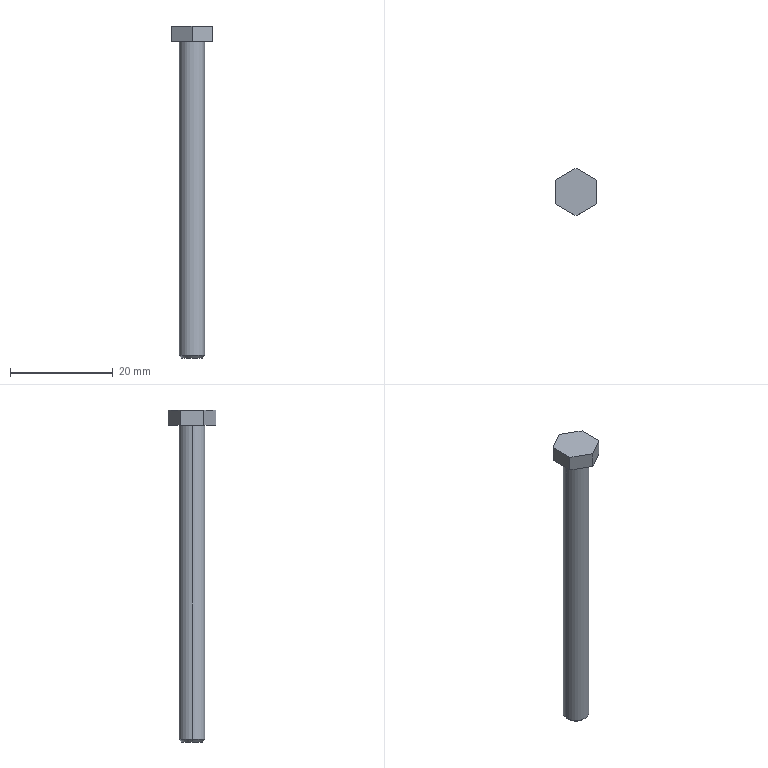Part | SolidWorks | features BaseBody 1 | 1 solid | 13 faces | box 8 x 9.238 x 64.5 mm | volume 1372 mm3 | plane 9 | cylinder 2 | cone 2 | commonest cylinder face diameters 5 x2
STEP:
#1=CARTESIAN_POINT('',(-2.5,0.,30.75));
#2=VERTEX_POINT('',#1);
#3=CARTESIAN_POINT('',(2.5,0.,30.75));
#4=VERTEX_POINT('',#3);
#5=CARTESIAN_POINT('',(0.,0.,30.75));
#6=DIRECTION('',(0.,0.,-1.));
#7=DIRECTION('',(-1.,0.,0.));
#8=AXIS2_PLACEMENT_3D('',#5,#6,#7);
#9=CIRCLE('',#8,2.5);
#10=EDGE_CURVE('',#2,#4,#9,.T.);
#11=ORIENTED_EDGE('',*,*,#10,.T.);
#12=CARTESIAN_POINT('',(2.5,0.,-30.25));
#13=VERTEX_POINT('',#12);
#14=CARTESIAN_POINT('',(2.5,0.,30.75));
#15=DIRECTION('',(0.,0.,-1.));
#16=VECTOR('',#15,1000.);
#17=LINE('',#14,#16);
#18=EDGE_CURVE('',#4,#13,#17,.T.);
#19=ORIENTED_EDGE('',*,*,#18,.T.);
#20=CARTESIAN_POINT('',(-2.5,0.,-30.25));
#21=VERTEX_POINT('',#20);
#22=CARTESIAN_POINT('',(0.,0.,-30.25));
#23=DIRECTION('',(0.,0.,1.));
#24=DIRECTION('',(-1.,0.,0.));
#25=AXIS2_PLACEMENT_3D('',#22,#23,#24);
#26=CIRCLE('',#25,2.5);
#27=EDGE_CURVE('',#13,#21,#26,.T.);
#28=ORIENTED_EDGE('',*,*,#27,.T.);
#29=CARTESIAN_POINT('',(-2.5,0.,30.75));
#30=DIRECTION('',(0.,0.,-1.));
#31=VECTOR('',#30,1000.);
#32=LINE('',#29,#31);
#33=EDGE_CURVE('',#2,#21,#32,.T.);
#34=ORIENTED_EDGE('',*,*,#33,.F.);
#35=EDGE_LOOP('',(#11,#19,#28,#34));
#36=FACE_OUTER_BOUND('',#35,.T.);
#37=CARTESIAN_POINT('',(0.,0.,30.75));
#38=DIRECTION('',(0.,0.,-1.));
#39=DIRECTION('',(-1.,0.,0.));
#40=AXIS2_PLACEMENT_3D('',#37,#38,#39);
#41=CYLINDRICAL_SURFACE('',#40,2.5);
#42=ADVANCED_FACE('',(#36),#41,.T.);
#43=CARTESIAN_POINT('',(2.,0.,-30.75));
#44=VERTEX_POINT('',#43);
#45=CARTESIAN_POINT('',(-2.,0.,-30.75));
#46=VERTEX_POINT('',#45);
#47=CARTESIAN_POINT('',(0.,0.,-30.75));
#48=DIRECTION('',(0.,0.,1.));
#49=DIRECTION('',(1.,0.,0.));
#50=AXIS2_PLACEMENT_3D('',#47,#48,#49);
#51=CIRCLE('',#50,2.);
#52=EDGE_CURVE('',#44,#46,#51,.T.);
#53=ORIENTED_EDGE('',*,*,#52,.T.);
#54=CARTESIAN_POINT('',(-2.5,0.,-30.25));
#55=DIRECTION('',(-0.7071,0.,0.7071));
#56=VECTOR('',#55,1000.);
#57=LINE('',#54,#56);
#58=EDGE_CURVE('',#46,#21,#57,.T.);
#59=ORIENTED_EDGE('',*,*,#58,.T.);
#60=ORIENTED_EDGE('',*,*,#27,.F.);
#61=CARTESIAN_POINT('',(2.5,0.,-30.25));
#62=DIRECTION('',(0.7071,0.,0.7071));
#63=VECTOR('',#62,1000.);
#64=LINE('',#61,#63);
#65=EDGE_CURVE('',#44,#13,#64,.T.);
#66=ORIENTED_EDGE('',*,*,#65,.F.);
#67=EDGE_LOOP('',(#53,#59,#60,#66));
#68=FACE_OUTER_BOUND('',#67,.T.);
#69=CARTESIAN_POINT('',(0.,0.,-30.25));
#70=DIRECTION('',(0.,0.,1.));
#71=DIRECTION('',(1.,0.,0.));
#72=AXIS2_PLACEMENT_3D('',#69,#70,#71);
#73=CONICAL_SURFACE('',#72,2.5,0.7854);
#74=ADVANCED_FACE('',(#68),#73,.T.);
#75=ORIENTED_EDGE('',*,*,#18,.F.);
#76=CARTESIAN_POINT('',(0.,0.,30.75));
#77=DIRECTION('',(0.,0.,-1.));
#78=DIRECTION('',(-1.,0.,0.));
#79=AXIS2_PLACEMENT_3D('',#76,#77,#78);
#80=CIRCLE('',#79,2.5);
#81=EDGE_CURVE('',#4,#2,#80,.T.);
#82=ORIENTED_EDGE('',*,*,#81,.T.);
#83=ORIENTED_EDGE('',*,*,#33,.T.);
#84=CARTESIAN_POINT('',(0.,0.,-30.25));
#85=DIRECTION('',(0.,0.,1.));
#86=DIRECTION('',(-1.,0.,0.));
#87=AXIS2_PLACEMENT_3D('',#84,#85,#86);
#88=CIRCLE('',#87,2.5);
#89=EDGE_CURVE('',#21,#13,#88,.T.);
#90=ORIENTED_EDGE('',*,*,#89,.T.);
#91=EDGE_LOOP('',(#75,#82,#83,#90));
#92=FACE_OUTER_BOUND('',#91,.T.);
#93=CARTESIAN_POINT('',(0.,0.,30.75));
#94=DIRECTION('',(0.,0.,-1.));
#95=DIRECTION('',(-1.,0.,0.));
#96=AXIS2_PLACEMENT_3D('',#93,#94,#95);
#97=CYLINDRICAL_SURFACE('',#96,2.5);
#98=ADVANCED_FACE('',(#92),#97,.T.);
#99=ORIENTED_EDGE('',*,*,#58,.F.);
#100=CARTESIAN_POINT('',(0.,0.,-30.75));
#101=DIRECTION('',(0.,0.,1.));
#102=DIRECTION('',(1.,0.,0.));
#103=AXIS2_PLACEMENT_3D('',#100,#101,#102);
#104=CIRCLE('',#103,2.);
#105=EDGE_CURVE('',#46,#44,#104,.T.);
#106=ORIENTED_EDGE('',*,*,#105,.T.);
#107=ORIENTED_EDGE('',*,*,#65,.T.);
#108=ORIENTED_EDGE('',*,*,#89,.F.);
#109=EDGE_LOOP('',(#99,#106,#107,#108));
#110=FACE_OUTER_BOUND('',#109,.T.);
#111=CARTESIAN_POINT('',(0.,0.,-30.25));
#112=DIRECTION('',(0.,0.,1.));
#113=DIRECTION('',(1.,0.,0.));
#114=AXIS2_PLACEMENT_3D('',#111,#112,#113);
#115=CONICAL_SURFACE('',#114,2.5,0.7854);
#116=ADVANCED_FACE('',(#110),#115,.T.);
#117=CARTESIAN_POINT('',(0.,-4.619,30.75));
#118=VERTEX_POINT('',#117);
#119=CARTESIAN_POINT('',(4.,-2.309,30.75));
#120=VERTEX_POINT('',#119);
#121=CARTESIAN_POINT('',(0.,-4.619,30.75));
#122=DIRECTION('',(0.866,0.5,0.));
#123=VECTOR('',#122,1000.);
#124=LINE('',#121,#123);
#125=EDGE_CURVE('',#118,#120,#124,.T.);
#126=ORIENTED_EDGE('',*,*,#125,.F.);
#127=CARTESIAN_POINT('',(-4.,-2.309,30.75));
#128=VERTEX_POINT('',#127);
#129=CARTESIAN_POINT('',(-4.,-2.309,30.75));
#130=DIRECTION('',(0.866,-0.5,0.));
#131=VECTOR('',#130,1000.);
#132=LINE('',#129,#131);
#133=EDGE_CURVE('',#128,#118,#132,.T.);
#134=ORIENTED_EDGE('',*,*,#133,.F.);
#135=CARTESIAN_POINT('',(-4.,2.309,30.75));
#136=VERTEX_POINT('',#135);
#137=CARTESIAN_POINT('',(-4.,0.,30.75));
#138=DIRECTION('',(0.,-1.,0.));
#139=VECTOR('',#138,1000.);
#140=LINE('',#137,#139);
#141=EDGE_CURVE('',#136,#128,#140,.T.);
#142=ORIENTED_EDGE('',*,*,#141,.F.);
#143=CARTESIAN_POINT('',(0.,4.619,30.75));
#144=VERTEX_POINT('',#143);
#145=CARTESIAN_POINT('',(0.,4.619,30.75));
#146=DIRECTION('',(-0.866,-0.5,0.));
#147=VECTOR('',#146,1000.);
#148=LINE('',#145,#147);
#149=EDGE_CURVE('',#144,#136,#148,.T.);
#150=ORIENTED_EDGE('',*,*,#149,.F.);
#151=CARTESIAN_POINT('',(4.,2.309,30.75));
#152=VERTEX_POINT('',#151);
#153=CARTESIAN_POINT('',(4.,2.309,30.75));
#154=DIRECTION('',(-0.866,0.5,0.));
#155=VECTOR('',#154,1000.);
#156=LINE('',#153,#155);
#157=EDGE_CURVE('',#152,#144,#156,.T.);
#158=ORIENTED_EDGE('',*,*,#157,.F.);
#159=CARTESIAN_POINT('',(4.,0.,30.75));
#160=DIRECTION('',(0.,1.,0.));
#161=VECTOR('',#160,1000.);
#162=LINE('',#159,#161);
#163=EDGE_CURVE('',#120,#152,#162,.T.);
#164=ORIENTED_EDGE('',*,*,#163,.F.);
#165=EDGE_LOOP('',(#126,#134,#142,#150,#158,#164));
#166=FACE_OUTER_BOUND('',#165,.T.);
#167=ORIENTED_EDGE('',*,*,#10,.F.);
#168=ORIENTED_EDGE('',*,*,#81,.F.);
#169=EDGE_LOOP('',(#167,#168));
#170=FACE_BOUND('',#169,.T.);
#171=CARTESIAN_POINT('',(0.,0.,30.75));
#172=DIRECTION('',(0.,0.,1.));
#173=DIRECTION('',(1.,0.,0.));
#174=AXIS2_PLACEMENT_3D('',#171,#172,#173);
#175=PLANE('',#174);
#176=ADVANCED_FACE('',(#166,#170),#175,.F.);
#177=ORIENTED_EDGE('',*,*,#52,.F.);
#178=ORIENTED_EDGE('',*,*,#105,.F.);
#179=EDGE_LOOP('',(#177,#178));
#180=FACE_OUTER_BOUND('',#179,.T.);
#181=CARTESIAN_POINT('',(0.,0.,-30.75));
#182=DIRECTION('',(0.,0.,1.));
#183=DIRECTION('',(1.,0.,0.));
#184=AXIS2_PLACEMENT_3D('',#181,#182,#183);
#185=PLANE('',#184);
#186=ADVANCED_FACE('',(#180),#185,.F.);
#187=CARTESIAN_POINT('',(4.,-2.309,33.75));
#188=VERTEX_POINT('',#187);
#189=CARTESIAN_POINT('',(4.,2.309,33.75));
#190=VERTEX_POINT('',#189);
#191=CARTESIAN_POINT('',(4.,-2.309,33.75));
#192=DIRECTION('',(0.,1.,0.));
#193=VECTOR('',#192,1000.);
#194=LINE('',#191,#193);
#195=EDGE_CURVE('',#188,#190,#194,.T.);
#196=ORIENTED_EDGE('',*,*,#195,.F.);
#197=CARTESIAN_POINT('',(4.,-2.309,33.75));
#198=DIRECTION('',(0.,0.,1.));
#199=VECTOR('',#198,1000.);
#200=LINE('',#197,#199);
#201=EDGE_CURVE('',#120,#188,#200,.T.);
#202=ORIENTED_EDGE('',*,*,#201,.F.);
#203=ORIENTED_EDGE('',*,*,#163,.T.);
#204=CARTESIAN_POINT('',(4.,2.309,33.75));
#205=DIRECTION('',(0.,0.,-1.));
#206=VECTOR('',#205,1000.);
#207=LINE('',#204,#206);
#208=EDGE_CURVE('',#190,#152,#207,.T.);
#209=ORIENTED_EDGE('',*,*,#208,.F.);
#210=EDGE_LOOP('',(#196,#202,#203,#209));
#211=FACE_OUTER_BOUND('',#210,.T.);
#212=CARTESIAN_POINT('',(4.,-2.309,33.75));
#213=DIRECTION('',(-1.,0.,0.));
#214=DIRECTION('',(0.,-1.,0.));
#215=AXIS2_PLACEMENT_3D('',#212,#213,#214);
#216=PLANE('',#215);
#217=ADVANCED_FACE('',(#211),#216,.F.);
#218=CARTESIAN_POINT('',(0.,-4.619,33.75));
#219=VERTEX_POINT('',#218);
#220=CARTESIAN_POINT('',(0.,-4.619,33.75));
#221=DIRECTION('',(0.866,0.5,0.));
#222=VECTOR('',#221,1000.);
#223=LINE('',#220,#222);
#224=EDGE_CURVE('',#219,#188,#223,.T.);
#225=ORIENTED_EDGE('',*,*,#224,.F.);
#226=CARTESIAN_POINT('',(0.,-4.619,33.75));
#227=DIRECTION('',(0.,0.,1.));
#228=VECTOR('',#227,1000.);
#229=LINE('',#226,#228);
#230=EDGE_CURVE('',#118,#219,#229,.T.);
#231=ORIENTED_EDGE('',*,*,#230,.F.);
#232=ORIENTED_EDGE('',*,*,#125,.T.);
#233=ORIENTED_EDGE('',*,*,#201,.T.);
#234=EDGE_LOOP('',(#225,#231,#232,#233));
#235=FACE_OUTER_BOUND('',#234,.T.);
#236=CARTESIAN_POINT('',(0.,-4.619,33.75));
#237=DIRECTION('',(-0.5,0.866,0.));
#238=DIRECTION('',(-0.866,-0.5,0.));
#239=AXIS2_PLACEMENT_3D('',#236,#237,#238);
#240=PLANE('',#239);
#241=ADVANCED_FACE('',(#235),#240,.F.);
#242=CARTESIAN_POINT('',(-4.,-2.309,33.75));
#243=VERTEX_POINT('',#242);
#244=CARTESIAN_POINT('',(-4.,-2.309,33.75));
#245=DIRECTION('',(0.866,-0.5,0.));
#246=VECTOR('',#245,1000.);
#247=LINE('',#244,#246);
#248=EDGE_CURVE('',#243,#219,#247,.T.);
#249=ORIENTED_EDGE('',*,*,#248,.F.);
#250=CARTESIAN_POINT('',(-4.,-2.309,33.75));
#251=DIRECTION('',(0.,0.,1.));
#252=VECTOR('',#251,1000.);
#253=LINE('',#250,#252);
#254=EDGE_CURVE('',#128,#243,#253,.T.);
#255=ORIENTED_EDGE('',*,*,#254,.F.);
#256=ORIENTED_EDGE('',*,*,#133,.T.);
#257=ORIENTED_EDGE('',*,*,#230,.T.);
#258=EDGE_LOOP('',(#249,#255,#256,#257));
#259=FACE_OUTER_BOUND('',#258,.T.);
#260=CARTESIAN_POINT('',(-4.,-2.309,33.75));
#261=DIRECTION('',(0.5,0.866,0.));
#262=DIRECTION('',(-0.866,0.5,0.));
#263=AXIS2_PLACEMENT_3D('',#260,#261,#262);
#264=PLANE('',#263);
#265=ADVANCED_FACE('',(#259),#264,.F.);
#266=CARTESIAN_POINT('',(-4.,2.309,33.75));
#267=VERTEX_POINT('',#266);
#268=CARTESIAN_POINT('',(-4.,2.309,33.75));
#269=DIRECTION('',(0.,-1.,0.));
#270=VECTOR('',#269,1000.);
#271=LINE('',#268,#270);
#272=EDGE_CURVE('',#267,#243,#271,.T.);
#273=ORIENTED_EDGE('',*,*,#272,.F.);
#274=CARTESIAN_POINT('',(-4.,2.309,33.75));
#275=DIRECTION('',(0.,0.,1.));
#276=VECTOR('',#275,1000.);
#277=LINE('',#274,#276);
#278=EDGE_CURVE('',#136,#267,#277,.T.);
#279=ORIENTED_EDGE('',*,*,#278,.F.);
#280=ORIENTED_EDGE('',*,*,#141,.T.);
#281=ORIENTED_EDGE('',*,*,#254,.T.);
#282=EDGE_LOOP('',(#273,#279,#280,#281));
#283=FACE_OUTER_BOUND('',#282,.T.);
#284=CARTESIAN_POINT('',(-4.,2.309,33.75));
#285=DIRECTION('',(1.,0.,0.));
#286=DIRECTION('',(0.,0.,-1.));
#287=AXIS2_PLACEMENT_3D('',#284,#285,#286);
#288=PLANE('',#287);
#289=ADVANCED_FACE('',(#283),#288,.F.);
#290=CARTESIAN_POINT('',(0.,4.619,33.75));
#291=VERTEX_POINT('',#290);
#292=CARTESIAN_POINT('',(0.,4.619,33.75));
#293=DIRECTION('',(-0.866,-0.5,0.));
#294=VECTOR('',#293,1000.);
#295=LINE('',#292,#294);
#296=EDGE_CURVE('',#291,#267,#295,.T.);
#297=ORIENTED_EDGE('',*,*,#296,.F.);
#298=CARTESIAN_POINT('',(0.,4.619,33.75));
#299=DIRECTION('',(0.,0.,1.));
#300=VECTOR('',#299,1000.);
#301=LINE('',#298,#300);
#302=EDGE_CURVE('',#144,#291,#301,.T.);
#303=ORIENTED_EDGE('',*,*,#302,.F.);
#304=ORIENTED_EDGE('',*,*,#149,.T.);
#305=ORIENTED_EDGE('',*,*,#278,.T.);
#306=EDGE_LOOP('',(#297,#303,#304,#305));
#307=FACE_OUTER_BOUND('',#306,.T.);
#308=CARTESIAN_POINT('',(0.,4.619,33.75));
#309=DIRECTION('',(0.5,-0.866,0.));
#310=DIRECTION('',(0.866,0.5,0.));
#311=AXIS2_PLACEMENT_3D('',#308,#309,#310);
#312=PLANE('',#311);
#313=ADVANCED_FACE('',(#307),#312,.F.);
#314=CARTESIAN_POINT('',(4.,2.309,33.75));
#315=DIRECTION('',(-0.866,0.5,0.));
#316=VECTOR('',#315,1000.);
#317=LINE('',#314,#316);
#318=EDGE_CURVE('',#190,#291,#317,.T.);
#319=ORIENTED_EDGE('',*,*,#318,.F.);
#320=ORIENTED_EDGE('',*,*,#208,.T.);
#321=ORIENTED_EDGE('',*,*,#157,.T.);
#322=ORIENTED_EDGE('',*,*,#302,.T.);
#323=EDGE_LOOP('',(#319,#320,#321,#322));
#324=FACE_OUTER_BOUND('',#323,.T.);
#325=CARTESIAN_POINT('',(4.,2.309,33.75));
#326=DIRECTION('',(-0.5,-0.866,0.));
#327=DIRECTION('',(0.866,-0.5,0.));
#328=AXIS2_PLACEMENT_3D('',#325,#326,#327);
#329=PLANE('',#328);
#330=ADVANCED_FACE('',(#324),#329,.F.);
#331=ORIENTED_EDGE('',*,*,#272,.T.);
#332=ORIENTED_EDGE('',*,*,#248,.T.);
#333=ORIENTED_EDGE('',*,*,#224,.T.);
#334=ORIENTED_EDGE('',*,*,#195,.T.);
#335=ORIENTED_EDGE('',*,*,#318,.T.);
#336=ORIENTED_EDGE('',*,*,#296,.T.);
#337=EDGE_LOOP('',(#331,#332,#333,#334,#335,#336));
#338=FACE_OUTER_BOUND('',#337,.T.);
#339=CARTESIAN_POINT('',(0.,0.,33.75));
#340=DIRECTION('',(0.,0.,1.));
#341=DIRECTION('',(1.,0.,0.));
#342=AXIS2_PLACEMENT_3D('',#339,#340,#341);
#343=PLANE('',#342);
#344=ADVANCED_FACE('',(#338),#343,.T.);
#345=CLOSED_SHELL('',(#42,#74,#98,#116,#176,#186,#217,#241,#265,#289,#313,#330,#344));
#346=MANIFOLD_SOLID_BREP('',#345);
#347=CARTESIAN_POINT('',(0.,0.,0.));
#348=DIRECTION('',(0.,0.,1.));
#349=DIRECTION('',(1.,0.,0.));
#350=AXIS2_PLACEMENT_3D('',#347,#348,#349);
#351=(LENGTH_UNIT()NAMED_UNIT(*)SI_UNIT(.MILLI.,.METRE.));
#352=UNCERTAINTY_MEASURE_WITH_UNIT(LENGTH_MEASURE(0.00001),#351,'','');
#353=(NAMED_UNIT(*)PLANE_ANGLE_UNIT()SI_UNIT($,.RADIAN.));
#354=(NAMED_UNIT(*)SI_UNIT($,.STERADIAN.)SOLID_ANGLE_UNIT());
#355=(GEOMETRIC_REPRESENTATION_CONTEXT(3)GLOBAL_UNCERTAINTY_ASSIGNED_CONTEXT((#352))GLOBAL_UNIT_ASSIGNED_CONTEXT((#351,#353,#354))REPRESENTATION_CONTEXT('',''));
#356=ADVANCED_BREP_SHAPE_REPRESENTATION('',(#346,#350),#355);